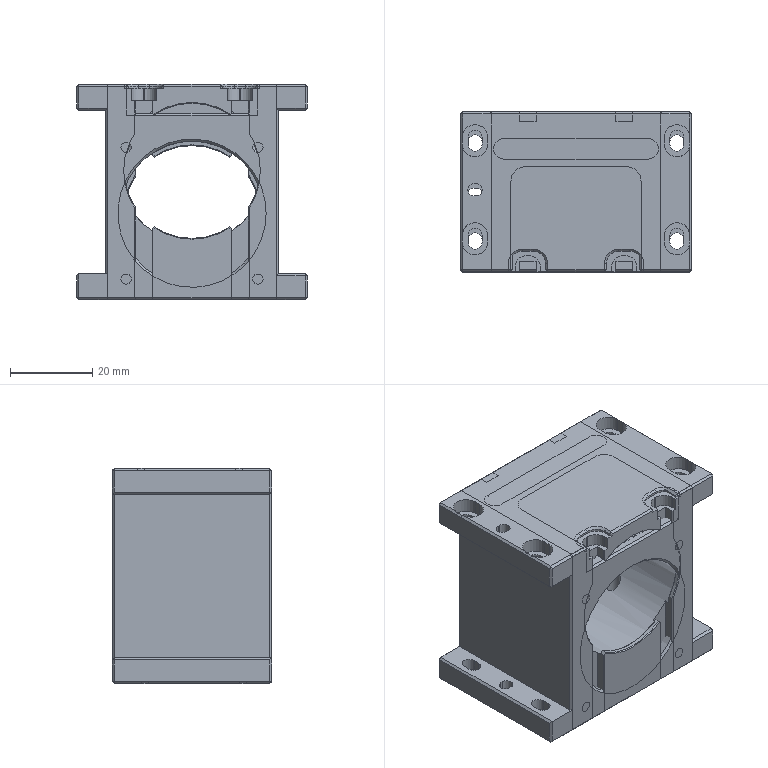NC program | NX | posted with a generic post | part box 56 x 38.8 x 52.3 mm
Whole program:
N10 G17 G21 G94 G90
(外形动态铣_1 , TOOL : 粗刀D10)
N12 T15 M6
N14 G54
N16 G17 G0 G90 X-37.859 Y-0.772 S8500 M3
N18 G43 Z27.7 H15
N20 G94 G1 Z3.1 F5000.
N22 Z0.1 F1300.
N24 X-35.751 Y-0.435 F4500.
N26 G3 X-35.094 Y-0.031 R1.01
N28 X-34.43 Y1.169 R3.982
N30 X-33.925 Y3.367 R11.529
N32 X-33.617 Y7.191 R37.37
N34 X-33.508 Y13.888 R191.307
N36 G2 X-33.493 Y20.075 R864.162
N38 X-33.267 Y21.553 R5.319
N40 X-32.543 Y22.856 R3.652
N42 X-31.38 Y23.897 R5.732
N44 X-29.19 Y24.95 R8.686
N46 X-25.89 Y25.631 R17.273
N48 X-21.213 Y25.924 R54.136
N50 X-12.214 Y25.999 R370.104
N52 G1 X27.474 Y25.995
N54 G2 X28.958 Y25.805 R6.121
N56 X30.421 Y24.989 R4.076
N58 X31.805 Y23.209 R6.135
N60 X32.669 Y20.937 R10.19
N62 X33.229 Y17.423 R21.613
N64 X33.442 Y12.928 R64.36
N66 X33.499 Y4.679 R428.413
N68 G1 X33.498 Y-19.821
N70 G2 X33.291 Y-21.491 R6.502
N72 X32.216 Y-23.225 R4.024
N74 X30.535 Y-24.405 R6.526
N76 X27.503 Y-25.384 R11.785
N78 X24.155 Y-25.791 R27.909
N80 X19.283 Y-25.963 R86.942
N82 X8.971 Y-26. R833.693
N84 G1 X-27.341 Y-25.998
N86 G2 X-28.828 Y-25.829 R6.279
N88 X-30.172 Y-25.188 R3.523
N90 X-31.446 Y-23.826 R5.205
N92 X-32.474 Y-21.624 R8.886
N94 X-33.118 Y-18.507 R17.227
N96 X-33.41 Y-14.206 R49.04
N98 X-33.499 Y-5.77 R297.961
N100 X-33.49 Y-3.52 R88.33
N102 X-33.219 Y-1.288 R17.834
N104 G3 X-32.613 Y2.397 R103.419
N106 X-32.124 Y8.685 R63.724
N108 X-32.004 Y17.258 R277.923
N110 G2 X-30.909 Y20.575 R5.169
N112 X-28.623 Y22.486 R7.403
N114 X-25.466 Y23.653 R12.635
N116 X-21.76 Y24.204 R26.322
N118 X-16.704 Y24.442 R75.166
N120 X-6.017 Y24.499 R594.696
N122 G1 X24.858 Y24.498
N124 G2 X28.006 Y23.459 R5.144
N126 X29.651 Y21.678 R6.908
N128 X30.771 Y19.306 R9.963
N130 X31.507 Y16.017 R18.056
N132 X31.864 Y11.721 R45.31
N134 X31.977 Y6.847 R137.853
N136 X32. Y-1.157 R663.719
N138 G1 X31.998 Y-17.407
N140 G2 X30.93 Y-20.545 R5.124
N142 X29.561 Y-21.883 R6.64
N144 X27.252 Y-23.114 R9.478
N146 X23.428 Y-24.023 R17.694
N148 X18.569 Y-24.391 R50.772
N150 X10.508 Y-24.499 R274.793
N152 G1 X-24.867 Y-24.497
N154 G2 X-28.164 Y-23.342 R5.199
N156 X-29.665 Y-21.664 R7.038
N158 X-30.945 Y-18.751 R10.853
N160 X-31.646 Y-14.881 R21.793
N162 X-31.928 Y-9.828 R63.677
N164 X-31.973 Y-5.704 R109.054
N166 X-31.671 Y-1.967 R36.841
N168 G3 X-31.132 Y2.308 R320.197
N170 X-30.602 Y10.545 R97.297
N172 X-30.52 Y14.993 R322.468
N174 G2 X-29.862 Y17.703 R6.334
N176 X-27.812 Y20.108 R6.989
N178 X-24.824 Y21.646 R10.656
N180 X-21.172 Y22.474 R20.032
N182 X-16.502 Y22.861 R49.488
N184 X-11.066 Y22.979 R154.867
N186 X-3.941 Y22.999 R662.121
N188 G1 X22.434 Y22.996
N190 G2 X25.321 Y22.29 R6.318
N192 X27.573 Y20.336 R7.064
N194 X28.933 Y17.881 R10.131
N196 X29.881 Y14.26 R17.893
N198 X30.358 Y9.035 R45.576
N200 X30.487 Y2.849 R163.833
N202 G1 X30.5 Y-2.026
N204 Y-14.526
N206 G2 X30.279 Y-16.571 R8.081
N208 X28.164 Y-19.821 R6.511
N210 X25.769 Y-21.277 R9.323
N212 X22.359 Y-22.28 R16.208
N214 X17.703 Y-22.8 R37.273
N216 X11.519 Y-22.977 R129.016
N218 X3.269 Y-22.999 R949.765
N220 G1 X-22.356 Y-22.997
N222 G2 X-24.563 Y-22.621 R6.645
N224 X-27.164 Y-20.835 R6.495
N226 X-28.834 Y-18.134 R9.201
N228 X-29.773 Y-14.899 R16.29
N230 X-30.309 Y-10.057 R37.442
N232 X-30.193 Y-3.128 R43.468
N234 X-29.689 Y1.747 R346.412
N236 G3 X-29.112 Y11.134 R123.315
N238 G2 X-29.035 Y13.195 R37.454
N240 X-28.378 Y15.722 R7.29
N242 X-25.817 Y18.654 R7.6
N244 X-22.964 Y20.063 R11.537
N246 X-19.316 Y20.914 R20.968
N248 X-14.275 Y21.351 R49.166
N250 X-7.151 Y21.489 R200.212
N252 G1 X-2.089 Y21.499
N254 X19.974 Y21.495
N256 G2 X21.835 Y21.303 R9.001
N258 X25.35 Y19.263 R6.891
N260 X27.015 Y16.783 R9.456
N262 X28.08 Y13.587 R15.457
N264 X28.691 Y9.322 R31.434
N266 X28.94 Y3.891 R87.2
N268 X28.999 Y-4.921 R453.699
N270 G1 X28.994 Y-12.546
N272 G2 X28.576 Y-15.126 R8.329
N274 X26.255 Y-18.294 R7.078
N276 X23.301 Y-19.93 R10.781
N278 X19.673 Y-20.853 R19.403
N280 X14.449 Y-21.343 R46.182
N282 X7.513 Y-21.488 R177.092
N284 G1 X2.638 Y-21.499
N286 X-19.987 Y-21.494
N288 G2 X-22.211 Y-21.206 R8.591
N290 X-25.359 Y-19.253 R6.962
N292 X-27.126 Y-16.531 R10.076
N294 X-28.283 Y-12.582 R16.947
N296 X-28.75 Y-6.609 R32.384
N298 X-28.537 Y-2.302 R59.609
N300 G3 X-28.017 Y3.734 R971.381
N302 X-27.643 Y10.559 R185.005
N304 G2 X-27.307 Y12.779 R10.278
N306 X-25.137 Y16.253 R7.38
N308 X-22.298 Y18.065 R10.318
N310 X-18.534 Y19.195 R17.416
N312 X-14.07 Y19.738 R38.211
N314 X-7.512 Y19.965 R118.376
N316 X-0.012 Y19.999 R559.44
N318 G1 X17.738 Y19.996
N320 G2 X19.972 Y19.773 R10.848
N322 X23.662 Y17.662 R7.337
N324 X25.591 Y14.689 R10.064
N326 X26.596 Y11.472 R16.685
N328 X27.232 Y6.643 R35.037
N330 X27.468 Y-0.102 R117.986
N332 X27.49 Y-10.47 R572.501
N334 X27.217 Y-12.698 R9.92
N336 X25.262 Y-16.06 R7.222
N338 X22.491 Y-17.956 R9.936
N340 X18.923 Y-19.107 R16.584
N342 X14.84 Y-19.678 R33.535
N344 X8.659 Y-19.948 R96.825
N346 X-0.22 Y-19.999 R453.121
N348 G1 X-17.782 Y-19.994
N350 G2 X-20.015 Y-19.759 R10.494
N352 X-23.426 Y-17.888 R7.348
N354 X-25.456 Y-14.985 R9.805
N356 X-26.598 Y-11.422 R15.8
N358 X-27.074 Y-6.577 R26.45
N360 X-26.88 Y-1.145 R64.933
N362 G3 X-26.447 Y4.801 R997.033
N364 G1 X-26.223 Y8.732
N366 G2 X-25.751 Y11.307 R10.334
N368 X-23.345 Y14.831 R7.954
N370 X-20.126 Y16.721 R11.131
N372 X-16.7 Y17.678 R18.784
N374 X-11.861 Y18.251 R40.176
N376 X-5.678 Y18.461 R125.452
N378 X1.072 Y18.498 R461.439
N380 G1 X15.447 Y18.496
N382 G2 X17.69 Y18.343 R14.739
N384 X22.204 Y15.869 R7.651
N386 X24.024 Y12.988 R10.634
N388 X25.085 Y9.587 R17.432
N390 X25.72 Y4.757 R36.204
N392 X25.964 Y-1.988 R118.498
N394 X25.989 Y-8.362 R288.442
N396 X25.804 Y-10.414 R12.008
N398 X23.479 Y-14.606 R7.673
N400 X20.964 Y-16.309 R10.198
N402 X17.239 Y-17.555 R16.626
N404 X13.345 Y-18.129 R33.046
N406 X7.729 Y-18.422 R84.092
N408 X-2.395 Y-18.499 R430.062
N410 G1 X-15.083
N412 G2 X-17.515 Y-18.371 R18.151
N414 X-22.095 Y-15.992 R7.699
N416 X-23.865 Y-13.326 R10.245
N418 X-25.046 Y-9.387 R15.426
N420 X-25.398 Y-4.906 R28.185
N422 X-25.279 Y-0.596 R67.14
N424 G1 X-24.836 Y6.662
N426 G2 X-24.411 Y9.247 R12.697
N428 X-21.775 Y13.264 R8.241
N430 X-18.73 Y15.084 R11.395
N432 X-14.767 Y16.201 R19.287
N434 X-9.552 Y16.774 R44.296
N436 X-2.993 Y16.971 R140.431
N438 X5.257 Y16.998 R800.548
N440 G1 X13.445 Y16.995
N442 G2 X15.875 Y16.837 R16.325
N444 X20.443 Y14.451 R7.932
N446 X22.403 Y11.495 R10.576
N448 X23.588 Y7.742 R17.92
N450 X24.239 Y2.537 R39.007
N452 X24.46 Y-3.646 R115.87
N454 X24.456 Y-7.021 R70.73
N456 X24.046 Y-9.606 R10.053
N458 X21.57 Y-13.291 R7.938
N460 X18.682 Y-15.04 R11.344
N462 X14.358 Y-16.25 R19.506
N464 X9.327 Y-16.782 R45.489
N466 X2.768 Y-16.972 R141.428
N468 X-4.17 Y-16.998 R569.74
N470 G1 X-13.482 Y-16.996
N472 G2 X-15.912 Y-16.831 R15.922
N474 X-20.719 Y-14.145 R7.891
N476 X-22.715 Y-10.564 R10.783
N478 X-23.496 Y-7.095 R17.348
N480 X-23.73 Y-2.229 R35.431
N482 X-23.421 Y4.888 R137.138
N484 X-22.995 Y7.474 R13.428
N486 X-20.145 Y11.785 R8.533
N488 X-16.884 Y13.648 R12.163
N490 X-12.722 Y14.748 R20.906
N492 X-7.877 Y15.264 R46.07
N494 X-1.693 Y15.462 R125.443
N496 X11.932 Y15.49 R984.409
N498 X14.543 Y15.256 R14.805
N500 X19.026 Y12.702 R8.188
N502 X20.933 Y9.7 R11.26
N504 X22.157 Y5.569 R18.898
N506 X22.735 Y0.731 R41.674
N508 X22.922 Y-4.89 R83.878
N510 X22.668 Y-7.31 R11.867
N512 X20.122 Y-11.588 R8.032
N514 X16.939 Y-13.54 R11.375
N516 X13.345 Y-14.603 R19.07
N518 X8.137 Y-15.239 R40.663
N520 X1.392 Y-15.465 R128.391
N522 X-11.969 Y-15.49 R958.377
N524 X-14.579 Y-15.251 R14.506
N526 X-19.275 Y-12.371 R7.956
N528 X-21.041 Y-9.084 R10.808
N530 X-21.848 Y-5.429 R18.018
N532 X-22.08 Y-0.375 R39.59
N534 X-21.946 Y3.372 R52.431
N536 X-21.442 Y6.132 R11.896
N538 X-18.749 Y10.12 R8.691
N540 X-15.696 Y11.959 R11.743
N542 X-11.929 Y13.081 R19.592
N544 X-6.722 Y13.724 R40.616
N546 X-0.352 Y13.955 R120.95
N548 X10.148 Y13.987 R533.487
N550 X12.391 Y13.831 R17.56
N552 X17.553 Y11.031 R8.376
N554 X19.357 Y8.184 R11.234
N556 X20.61 Y4.068 R18.785
N558 X21.213 Y-0.768 R40.377
N560 X21.299 Y-3.953 R29.817
N562 X20.728 Y-6.884 R9.097
N564 X18.478 Y-10.069 R8.216
N566 X15.272 Y-12.021 R11.427
N568 X11.864 Y-13.046 R19.279
N570 X7.035 Y-13.688 R37.979
N572 X-0.084 Y-13.96 R119.443
N574 X-10.209 Y-13.987 R497.63
N576 X-12.82 Y-13.756 R14.941
N578 X-17.437 Y-11.06 R7.911
N580 X-19.216 Y-7.994 R10.274
N582 X-20.099 Y-4.55 R16.797
N584 X-20.384 Y1.995 R32.803
N586 X-19.796 Y4.927 R10.705
N588 X-17.349 Y8.46 R8.642
N590 X-14.335 Y10.345 R11.746
N592 X-10.583 Y11.515 R18.883
N594 X-5.755 Y12.169 R38.256
N596 X1.175 Y12.451 R115.249
N598 X8.488 Y12.483 R287.975
N600 X10.915 Y12.29 R16.548
N602 X15.927 Y9.565 R8.48
N604 X17.995 Y6.211 R11.773
N606 X19.099 Y2.438 R19.79
N608 X19.601 Y-1.84 R26.712
N610 X19.302 Y-4.627 R9.493
N612 X16.955 Y-8.419 R7.942
N614 X13.797 Y-10.426 R11.216
N616 X9.669 Y-11.64 R19.419
N618 X4.831 Y-12.22 R42.977
N620 X-1.164 Y-12.448 R113.358
N622 X-8.664 Y-12.481 R269.894
N624 X-11.089 Y-12.261 R15.307
N626 X-15.953 Y-9.319 R7.992
N628 X-17.591 Y-6.369 R11.025
N630 X-18.538 Y-2.364 R17.498
N632 X-18.654 Y1.19 R16.923
N634 X-17.368 Y5.067 R8.555
N636 X-14.903 Y7.612 R9.123
N638 X-11.388 Y9.357 R13.613
N640 X-6.82 Y10.376 R24.686
N642 X-1.029 Y10.844 R60.99
N644 X6.844 Y10.97 R170.83
N646 X9.457 Y10.748 R16.818
N648 X14.556 Y7.818 R8.566
N650 X16.408 Y4.785 R11.593
N652 X17.724 Y-0.478 R17.481
N654 X17.375 Y-3.625 R8.107
N656 X15.356 Y-6.789 R7.791
N658 X12.719 Y-8.618 R10.592
N660 X8.81 Y-9.953 R17.237
N662 X4.735 Y-10.581 R34.305
N664 X-0.692 Y-10.896 R80.208
N666 X-7.066 Y-10.965 R147.564
N668 X-9.674 Y-10.697 R14.181
N670 X-14.096 Y-8.047 R7.971
N672 X-15.955 Y-4.811 R11.011
N674 X-16.771 Y-0.974 R13.153
N676 X-16.261 Y2.337 R8.112
N678 X-13.988 Y5.507 R8.264
N680 X-10.598 Y7.528 R11.955
N682 X-6.817 Y8.604 R20.336
N684 X-1.606 Y9.223 R43.264
N686 X5.326 Y9.435 R101.692
N688 X7.754 Y9.241 R16.49
N690 X11.968 Y7.324 R8.608
N692 X14.566 Y3.901 R10.623
N694 X15.53 Y1.067 R11.233
N696 X14.134 Y-4.57 R6.799
N698 X11.408 Y-6.843 R9.315
N700 X7.933 Y-8.226 R14.931
N702 X3.695 Y-9. R28.346
N704 X-2.291 Y-9.389 R72.6
N706 X-6.04 Y-9.408 R53.699
N708 X-8.628 Y-9.011 R10.81
N710 X-12.363 Y-6.611 R7.872
N712 X-14.403 Y-2.651 R9.146
N714 X-13.182 Y2.842 R6.615
N716 X-10.682 Y5.08 R8.992
N718 X-7.6 Y6.466 R13.931
N720 X-3.016 Y7.426 R26.092
N722 X4.091 Y7.856 R57.224
N724 X7.064 Y7.511 R12.978
N726 X11.801 Y4.315 R8.59
N728 X12.939 Y2.173 R7.378
N730 X12.538 Y-2.188 R5.559
N732 X10.338 Y-4.709 R7.458
N734 X7.337 Y-6.293 R11.755
N736 X3.711 Y-7.229 R20.785
N738 X-1.883 Y-7.794 R46.778
N740 X-4.694 Y-7.819 R28.809
N742 X-7.8 Y-7.177 R9.384
N744 X-10.985 Y-4.644 R7.241
N746 X-11.568 Y0.009 R5.055
N748 X-10.312 Y2.083 R6.394
N750 X-8.132 Y3.841 R8.987
N752 X-4.657 Y5.243 R14.425
N754 X-0.23 Y6.028 R28.201
N756 X3.325 Y6.199 R26.447
N758 X6.271 Y5.694 R10.201
N760 X8.702 Y4.313 R7.411
N762 X9.649 Y3.158 R4.603
N764 X10.165 Y0.813 R4.059
N766 X9.574 Y-1.148 R4.997
N768 X7.459 Y-3.494 R6.873
N770 X4.965 Y-4.807 R10.96
N772 X0.788 Y-5.847 R20.062
N774 X-2.946 Y-6.15 R24.978
N776 X-5.715 Y-5.727 R9.203
N778 X-7.201 Y-4.943 R5.092
N780 X-8.385 Y-2.482 R3.349
N782 X-7.895 Y-0.31 R4.529
N784 X-6.397 Y1.593 R6.186
N786 X-4.337 Y2.927 R9.092
N788 X-0.778 Y4.075 R14.846
N790 X2.576 Y4.378 R13.895
N792 X4.24 Y4.126 R7.653
N794 X5.836 Y2.432 R2.324
N796 X5.848 Y0.945 R3.351
N798 X5.087 Y-0.755 R4.628
N800 X3.178 Y-2.53 R6.538
N802 X0.08 Y-3.833 R10.443
N804 X-1.582 Y-4.111 R9.824
N806 X-2.105 Y-3.929 R0.903
N808 X-3.14 Y-2.402 R2.971
N810 X-3.276 Y-0.735 R3.758
N812 X-2.679 Y1.031 R4.969
N814 G1 Z3.1
N816 G0 Z27.7
N818 M5
(轮廓开粗_1_COPY , TOOL : 粗刀D4)
N820 T18 M6
N822 G54
N824 G17 G0 G90 X12.65 Y-22. S8000 M3
N826 G43 Z10. H18
N828 Z-0.281
N830 G41 G94 G1 Y-19.4 F1500. D18
N832 Y-18.4
N834 G3 X11.8 Y-17.55 R0.85
N836 G1 X11.6
N838 G3 X10.75 Y-18.4 R0.85
N840 G1 Y-19.4
N842 Y-21.8
N844 G40
N846 Y-22.
N848 G0 X12.65 Z-0.561
N850 G41 G1 Y-19.4
N852 Y-18.4
N854 G3 X11.8 Y-17.55 R0.85
N856 G1 X11.6
N858 G3 X10.75 Y-18.4 R0.85
N860 G1 Y-19.4
N862 Y-21.8
N864 G40
N866 Y-22.
N868 G0 X12.65 Z-0.842
N870 G41 G1 Y-19.4
N872 Y-18.4
N874 G3 X11.8 Y-17.55 R0.85
N876 G1 X11.6
N878 G3 X10.75 Y-18.4 R0.85
N880 G1 Y-19.4
N882 Y-21.8
N884 G40
N886 Y-22.
N888 G0 X12.65 Z-1.123
N890 G41 G1 Y-19.4
N892 Y-18.4
N894 G3 X11.8 Y-17.55 R0.85
N896 G1 X11.6
N898 G3 X10.75 Y-18.4 R0.85
N900 G1 Y-19.4
N902 Y-21.8
N904 G40
N906 Y-22.
N908 G0 X12.65 Z-1.404
N910 G41 G1 Y-19.4
N912 Y-18.4
N914 G3 X11.8 Y-17.55 R0.85
N916 G1 X11.6
N918 G3 X10.75 Y-18.4 R0.85
N920 G1 Y-19.4
N922 Y-21.8
N924 G40
N926 Y-22.
N928 G0 X12.65 Z-1.684
N930 G41 G1 Y-19.4
N932 Y-18.4
N934 G3 X11.8 Y-17.55 R0.85
N936 G1 X11.6
N938 G3 X10.75 Y-18.4 R0.85
N940 G1 Y-19.4
N942 Y-21.8
N944 G40
N946 Y-22.
N948 G0 X12.65 Z-1.965
N950 G41 G1 Y-19.4
N952 Y-18.4
N954 G3 X11.8 Y-17.55 R0.85
N956 G1 X11.6
N958 G3 X10.75 Y-18.4 R0.85
N960 G1 Y-19.4
N962 Y-21.8
N964 G40
N966 Y-22.
N968 G0 X12.65 Z-2.246
N970 G41 G1 Y-19.4
N972 Y-18.4
N974 G3 X11.8 Y-17.55 R0.85
N976 G1 X11.6
N978 G3 X10.75 Y-18.4 R0.85
N980 G1 Y-19.4
N982 Y-21.8
N984 G40
N986 Y-22.
N988 G0 X12.65 Z-2.526
N990 G41 G1 Y-19.4
N992 Y-18.4
N994 G3 X11.8 Y-17.55 R0.85
N996 G1 X11.6
N998 G3 X10.75 Y-18.4 R0.85
N1000 G1 Y-19.4
N1002 Y-21.8
N1004 G40
N1006 Y-22.
N1008 G0 X12.65 Z-2.807
N1010 G41 G1 Y-19.4
N1012 Y-18.4
N1014 G3 X11.8 Y-17.55 R0.85
N1016 G1 X11.6
N1018 G3 X10.75 Y-18.4 R0.85
N1020 G1 Y-19.4
N1022 Y-21.8
N1024 G40
N1026 Y-22.
N1028 G0 X12.65 Z-3.088
N1030 G41 G1 Y-19.4
N1032 Y-18.4
N1034 G3 X11.8 Y-17.55 R0.85
N1036 G1 X11.6
N1038 G3 X10.75 Y-18.4 R0.85
N1040 G1 Y-19.4
N1042 Y-21.8
N1044 G40
N1046 Y-22.
N1048 G0 X12.65 Z-3.369
N1050 G41 G1 Y-19.4
N1052 Y-18.4
N1054 G3 X11.8 Y-17.55 R0.85
N1056 G1 X11.6
N1058 G3 X10.75 Y-18.4 R0.85
N1060 G1 Y-19.4
N1062 Y-21.8
N1064 G40
N1066 Y-22.
N1068 G0 X12.65 Z-3.649
N1070 G41 G1 Y-19.4
N1072 Y-18.4
N1074 G3 X11.8 Y-17.55 R0.85
N1076 G1 X11.6
N1078 G3 X10.75 Y-18.4 R0.85
N1080 G1 Y-19.4
N1082 Y-21.8
N1084 G40
N1086 Y-22.
N1088 G0 X12.65 Z-3.93
N1090 G41 G1 Y-19.4
N1092 Y-18.4
N1094 G3 X11.8 Y-17.55 R0.85
N1096 G1 X11.6
N1098 G3 X10.75 Y-18.4 R0.85
N1100 G1 Y-19.4
N1102 Y-21.8
N1104 G40
N1106 Y-22.
N1108 G0 Z10.
N1110 X-10.75
N1112 Z-0.281
N1114 G41 G1 Y-19.4
N1116 Y-18.4
N1118 G3 X-11.6 Y-17.55 R0.85
N1120 G1 X-11.8
N1122 G3 X-12.65 Y-18.4 R0.85
N1124 G1 Y-19.4
N1126 Y-21.8
N1128 G40
N1130 Y-22.
N1132 G0 X-10.75 Z-0.561
N1134 G41 G1 Y-19.4
N1136 Y-18.4
N1138 G3 X-11.6 Y-17.55 R0.85
N1140 G1 X-11.8
N1142 G3 X-12.65 Y-18.4 R0.85
N1144 G1 Y-19.4
N1146 Y-21.8
N1148 G40
N1150 Y-22.
N1152 G0 X-10.75 Z-0.842
N1154 G41 G1 Y-19.4
N1156 Y-18.4
N1158 G3 X-11.6 Y-17.55 R0.85
N1160 G1 X-11.8
N1162 G3 X-12.65 Y-18.4 R0.85
N1164 G1 Y-19.4
N1166 Y-21.8
N1168 G40
N1170 Y-22.
N1172 G0 X-10.75 Z-1.123
N1174 G41 G1 Y-19.4
N1176 Y-18.4
N1178 G3 X-11.6 Y-17.55 R0.85
N1180 G1 X-11.8
N1182 G3 X-12.65 Y-18.4 R0.85
N1184 G1 Y-19.4
N1186 Y-21.8
N1188 G40
N1190 Y-22.
N1192 G0 X-10.75 Z-1.404
N1194 G41 G1 Y-19.4
N1196 Y-18.4
N1198 G3 X-11.6 Y-17.55 R0.85
N1200 G1 X-11.8
N1202 G3 X-12.65 Y-18.4 R0.85
N1204 G1 Y-19.4
N1206 Y-21.8
N1208 G40
N1210 Y-22.
N1212 G0 X-10.75 Z-1.684
N1214 G41 G1 Y-19.4
N1216 Y-18.4
N1218 G3 X-11.6 Y-17.55 R0.85
N1220 G1 X-11.8
N1222 G3 X-12.65 Y-18.4 R0.85
N1224 G1 Y-19.4
N1226 Y-21.8
N1228 G40
N1230 Y-22.
N1232 G0 X-10.75 Z-1.965
N1234 G41 G1 Y-19.4
N1236 Y-18.4
N1238 G3 X-11.6 Y-17.55 R0.85
N1240 G1 X-11.8
N1242 G3 X-12.65 Y-18.4 R0.85
N1244 G1 Y-19.4
N1246 Y-21.8
N1248 G40
N1250 Y-22.
N1252 G0 X-10.75 Z-2.246
N1254 G41 G1 Y-19.4
N1256 Y-18.4
N1258 G3 X-11.6 Y-17.55 R0.85
N1260 G1 X-11.8
N1262 G3 X-12.65 Y-18.4 R0.85
N1264 G1 Y-19.4
N1266 Y-21.8
N1268 G40
N1270 Y-22.
N1272 G0 X-10.75 Z-2.526
N1274 G41 G1 Y-19.4
N1276 Y-18.4
N1278 G3 X-11.6 Y-17.55 R0.85
N1280 G1 X-11.8
N1282 G3 X-12.65 Y-18.4 R0.85
N1284 G1 Y-19.4
N1286 Y-21.8
N1288 G40
N1290 Y-22.
N1292 G0 X-10.75 Z-2.807
N1294 G41 G1 Y-19.4
N1296 Y-18.4
N1298 G3 X-11.6 Y-17.55 R0.85
N1300 G1 X-11.8
N1302 G3 X-12.65 Y-18.4 R0.85
N1304 G1 Y-19.4
N1306 Y-21.8
N1308 G40
N1310 Y-22.
N1312 G0 X-10.75 Z-3.088
N1314 G41 G1 Y-19.4
N1316 Y-18.4
N1318 G3 X-11.6 Y-17.55 R0.85
N1320 G1 X-11.8
N1322 G3 X-12.65 Y-18.4 R0.85
N1324 G1 Y-19.4
N1326 Y-21.8
N1328 G40
N1330 Y-22.
N1332 G0 X-10.75 Z-3.369
N1334 G41 G1 Y-19.4
N1336 Y-18.4
N1338 G3 X-11.6 Y-17.55 R0.85
N1340 G1 X-11.8
N1342 G3 X-12.65 Y-18.4 R0.85
N1344 G1 Y-19.4
N1346 Y-21.8
N1348 G40
N1350 Y-22.
N1352 G0 X-10.75 Z-3.649
N1354 G41 G1 Y-19.4
N1356 Y-18.4
N1358 G3 X-11.6 Y-17.55 R0.85
N1360 G1 X-11.8
N1362 G3 X-12.65 Y-18.4 R0.85
N1364 G1 Y-19.4
N1366 Y-21.8
N1368 G40
N1370 Y-22.
N1372 G0 X-10.75 Z-3.93
N1374 G41 G1 Y-19.4
N1376 Y-18.4
N1378 G3 X-11.6 Y-17.55 R0.85
N1380 G1 X-11.8
N1382 G3 X-12.65 Y-18.4 R0.85
N1384 G1 Y-19.4
N1386 Y-21.8
N1388 G40
N1390 Y-22.
N1392 G0 Z10.
(轮廓开粗_1 , TOOL : 粗刀D4)
N1394 X16.818 Y-22.759
N1396 Z1.535
N1398 G1 Z-0.465
N1400 G41 X14.98 Y-20.92
N1402 X14.48 Y-20.42
N1404 G2 X13.85 Y-18.9 R2.15
N1406 G1 Y-17.4
N1408 G3 X13. Y-16.55 R0.85
N1410 G1 X10.4
N1412 G3 X9.55 Y-17.4 R0.85
N1414 G1 Y-18.9
N1416 G2 X8.92 Y-20.42 R2.15
N1418 G1 X8.42 Y-20.92
N1420 X6.723 Y-22.617
N1422 G40
N1424 X6.582 Y-22.759
N1426 Z1.535
N1428 G0 Z10.
N1430 X16.818
N1432 Z1.07
N1434 G1 Z-0.93
N1436 G41 X14.98 Y-20.92
N1438 X14.48 Y-20.42
N1440 G2 X13.85 Y-18.9 R2.15
N1442 G1 Y-17.4
N1444 G3 X13. Y-16.55 R0.85
N1446 G1 X10.4
N1448 G3 X9.55 Y-17.4 R0.85
N1450 G1 Y-18.9
N1452 G2 X8.92 Y-20.42 R2.15
N1454 G1 X8.42 Y-20.92
N1456 X6.723 Y-22.617
N1458 G40
N1460 X6.582 Y-22.759
N1462 Z1.07
N1464 G0 Z10.
N1466 X-6.582
N1468 Z1.535
N1470 G1 Z-0.465
N1472 G41 X-8.42 Y-20.92
N1474 X-8.92 Y-20.42
N1476 G2 X-9.55 Y-18.9 R2.15
N1478 G1 Y-17.4
N1480 G3 X-10.4 Y-16.55 R0.85
N1482 G1 X-13.
N1484 G3 X-13.85 Y-17.4 R0.85
N1486 G1 Y-18.9
N1488 G2 X-14.48 Y-20.42 R2.15
N1490 G1 X-14.98 Y-20.92
N1492 X-16.677 Y-22.617
N1494 G40
N1496 X-16.818 Y-22.759
N1498 Z1.535
N1500 G0 Z10.
N1502 X-6.582
N1504 Z1.07
N1506 G1 Z-0.93
N1508 G41 X-8.42 Y-20.92
N1510 X-8.92 Y-20.42
N1512 G2 X-9.55 Y-18.9 R2.15
N1514 G1 Y-17.4
N1516 G3 X-10.4 Y-16.55 R0.85
N1518 G1 X-13.
N1520 G3 X-13.85 Y-17.4 R0.85
N1522 G1 Y-18.9
N1524 G2 X-14.48 Y-20.42 R2.15
N1526 G1 X-14.98 Y-20.92
N1528 X-16.677 Y-22.617
N1530 G40
N1532 X-16.818 Y-22.759
N1534 Z1.07
N1536 G0 Z10.
N1538 M5
(飞顶面D50_1 , TOOL : 飞刀D50)
N1540 T20 M6
N1542 G54
N1544 G17 G0 G90 X58. Y0. S5500 M3
N1546 G43 Z10. H20
N1548 Z2.
N1550 G94 G1 Z0. F1200.
N1552 X53.
N1554 X-53.
N1556 X-58.
N1558 Z2.
N1560 G0 Z10.
N1562 M5
(单向轮廓精光_3 , TOOL : 光刀D4)
N1564 T07 M6
N1566 G54
N1568 G17 G0 G90 X17.497 Y-23.211 S8000 M3
N1570 G43 Z10. H7
N1572 Z2.
N1574 G94 G1 Z-1. F700.
N1576 G41 X15.093 Y-20.807 D7
N1578 X14.602 Y-20.316
N1580 G2 X14.01 Y-18.888 R2.02
N1582 G1 Y-17.4
N1584 G3 X13. Y-16.39 R1.01
N1586 G1 X10.4
N1588 G3 X9.39 Y-17.4 R1.01
N1590 G1 Y-18.888
N1592 G2 X8.798 Y-20.316 R2.02
N1594 G1 X8.307 Y-20.807
N1596 X6.044 Y-23.07
N1598 G40
N1600 X5.903 Y-23.211
N1602 Z2.
N1604 G0 Z10.
N1606 X17.511 Y-23.197
N1608 Z2.
N1610 G1 Z-1.
N1612 G41 X15.107 Y-20.793
N1614 X14.616 Y-20.302
N1616 G2 X14.03 Y-18.888 R2.
N1618 G1 Y-17.4
N1620 G3 X13. Y-16.37 R1.03
N1622 G1 X10.4
N1624 G3 X9.37 Y-17.4 R1.03
N1626 G1 Y-18.888
N1628 G2 X8.784 Y-20.302 R2.
N1630 G1 X8.293 Y-20.793
N1632 X6.03 Y-23.056
N1634 G40
N1636 X5.889 Y-23.197
N1638 Z2.
N1640 G0 Z10.
N1642 X-5.903 Y-23.211
N1644 Z2.
N1646 G1 Z-1.
N1648 G41 X-8.307 Y-20.807
N1650 X-8.798 Y-20.316
N1652 G2 X-9.39 Y-18.888 R2.02
N1654 G1 Y-17.4
N1656 G3 X-10.4 Y-16.39 R1.01
N1658 G1 X-13.
N1660 G3 X-14.01 Y-17.4 R1.01
N1662 G1 Y-18.888
N1664 G2 X-14.602 Y-20.316 R2.02
N1666 G1 X-15.093 Y-20.807
N1668 X-17.356 Y-23.07
N1670 G40
N1672 X-17.497 Y-23.211
N1674 Z2.
N1676 G0 Z10.
N1678 X-5.889 Y-23.197
N1680 Z2.
N1682 G1 Z-1.
N1684 G41 X-8.293 Y-20.793
N1686 X-8.784 Y-20.302
N1688 G2 X-9.37 Y-18.888 R2.
N1690 G1 Y-17.4
N1692 G3 X-10.4 Y-16.37 R1.03
N1694 G1 X-13.
N1696 G3 X-14.03 Y-17.4 R1.03
N1698 G1 Y-18.888
N1700 G2 X-14.616 Y-20.302 R2.
N1702 G1 X-15.107 Y-20.793
N1704 X-17.37 Y-23.056
N1706 G40
N1708 X-17.511 Y-23.197
N1710 Z2.
N1712 G0 Z10.
(单向轮廓精光_3_COPY , TOOL : 光刀D4)
N1714 X12.81 Y-22.8
N1716 Z-1.
N1718 G1 Z-4.
N1720 G41 Y-19.4
N1722 Y-18.4
N1724 G3 X11.8 Y-17.39 R1.01
N1726 G1 X11.6
N1728 G3 X10.59 Y-18.4 R1.01
N1730 G1 Y-19.4
N1732 Y-22.6
N1734 G40
N1736 Y-22.8
N1738 Z-1.
N1740 G0 Z10.
N1742 X12.83
N1744 Z-1.
N1746 G1 Z-4.
N1748 G41 Y-19.4
N1750 Y-18.4
N1752 G3 X11.8 Y-17.37 R1.03
N1754 G1 X11.6
N1756 G3 X10.57 Y-18.4 R1.03
N1758 G1 Y-19.4
N1760 Y-22.6
N1762 G40
N1764 Y-22.8
N1766 Z-1.
N1768 G0 Z10.
N1770 X-10.59
N1772 Z-1.
N1774 G1 Z-4.
N1776 G41 Y-19.4
N1778 Y-18.4
N1780 G3 X-11.6 Y-17.39 R1.01
N1782 G1 X-11.8
N1784 G3 X-12.81 Y-18.4 R1.01
N1786 G1 Y-19.4
N1788 Y-22.6
N1790 G40
N1792 Y-22.8
N1794 Z-1.
N1796 G0 Z10.
N1798 X-10.57
N1800 Z-1.
N1802 G1 Z-4.
N1804 G41 Y-19.4
N1806 Y-18.4
N1808 G3 X-11.6 Y-17.37 R1.03
N1810 G1 X-11.8
N1812 G3 X-12.83 Y-18.4 R1.03
N1814 G1 Y-19.4
N1816 Y-22.6
N1818 G40
N1820 Y-22.8
N1822 Z-1.
N1824 G0 Z10.
N1826 M5
(倒角刀D6._1 , TOOL : 倒角刀D6)
N1828 T11 M6
N1830 G54
N1832 G17 G0 G90 X-23.4 Y-0.6 S7500 M3
N1834 G43 Z10. H11
N1836 Z1.5
N1838 G94 G1 Z-1.5 F1200.
N1840 G41 X-22.6 D11
N1842 G3 X-22. Y0. R0.6
N1844 G1 Y18.693
N1846 G2 X-21.561 Y19.754 R1.5
N1848 G1 X-21.354 Y19.961
N1850 G2 X-20.293 Y20.4 R1.5
N1852 G1 X20.293
N1854 G2 X21.354 Y19.961 R1.5
N1856 G1 X21.561 Y19.754
N1858 G2 X22. Y18.693 R1.5
N1860 G1 Y-18.693
N1862 G2 X21.561 Y-19.754 R1.5
N1864 G1 X21.354 Y-19.961
N1866 G2 X20.293 Y-20.4 R1.5
N1868 G1 X-20.293
N1870 G2 X-21.354 Y-19.961 R1.5
N1872 G1 X-21.561 Y-19.754
N1874 G2 X-22. Y-18.693 R1.5
N1876 G1 Y0.
N1878 G3 X-22.6 Y0.6 R0.6
N1880 G1 X-23.2
N1882 G40
N1884 X-23.4
N1886 Z1.5
N1888 G0 Z10.
(倒角刀D6._1_COPY , TOOL : 倒角刀D6)
N1890 X-9.326 Y-23.069
N1892 Z-0.5
N1894 G1 Z-3.5
N1896 G41 X-8.826 Y-22.5
N1898 G3 X-8.88 Y-21.653 R0.6
N1900 G2 X-10.9 Y-19.2 R2.5
N1902 G1 Y-18.4
N1904 G3 X-11.6 Y-17.7 R0.7
N1906 G1 X-11.8
N1908 G3 X-12.5 Y-18.4 R0.7
N1910 G1 Y-19.2
N1912 G2 X-14.52 Y-21.653 R2.5
N1914 G3 X-14.574 Y-22.5 R0.6
N1916 G1 X-14.206 Y-22.918
N1918 G40
N1920 X-14.074 Y-23.069
N1922 Z-0.5
N1924 G0 Z10.
N1926 X14.074
N1928 Z-0.5
N1930 G1 Z-3.5
N1932 G41 X14.574 Y-22.5
N1934 G3 X14.52 Y-21.653 R0.6
N1936 G2 X12.5 Y-19.2 R2.5
N1938 G1 Y-18.4
N1940 G3 X11.8 Y-17.7 R0.7
N1942 G1 X11.6
N1944 G3 X10.9 Y-18.4 R0.7
N1946 G1 Y-19.2
N1948 G2 X8.88 Y-21.653 R2.5
N1950 G3 X8.826 Y-22.5 R0.6
N1952 G1 X9.194 Y-22.918
N1954 G40
N1956 X9.326 Y-23.069
N1958 Z-0.5
N1960 G0 Z10.
(倒角刀D6._1_COPY_1 , TOOL : 倒角刀D6)
N1962 X17.844 Y-21.309
N1964 Z2.1
N1966 G1 Z-0.9
N1968 G41 X16.217 Y-19.683
N1970 X15.864 Y-19.329
N1972 G2 X15.6 Y-18.693 R0.9
N1974 G1 Y-17.4
N1976 G3 X13. Y-14.8 R2.6
N1978 G1 X10.4
N1980 G3 X7.8 Y-17.4 R2.6
N1982 G1 Y-18.693
N1984 G2 X7.536 Y-19.329 R0.9
N1986 G1 X7.183 Y-19.683
N1988 X5.698 Y-21.168
N1990 G40
N1992 X5.556 Y-21.309
N1994 Z2.1
N1996 G0 Z10.
N1998 X-5.556
N2000 Z2.1
N2002 G1 Z-0.9
N2004 G41 X-7.183 Y-19.683
N2006 X-7.536 Y-19.329
N2008 G2 X-7.8 Y-18.693 R0.9
N2010 G1 Y-17.4
N2012 G3 X-10.4 Y-14.8 R2.6
N2014 G1 X-13.
N2016 G3 X-15.6 Y-17.4 R2.6
N2018 G1 Y-18.693
N2020 G2 X-15.864 Y-19.329 R0.9
N2022 G1 X-16.217 Y-19.683
N2024 X-17.702 Y-21.168
N2026 G40
N2028 X-17.844 Y-21.309
N2030 Z2.1
N2032 G0 Z10.
N2034 M5
N2036 M2